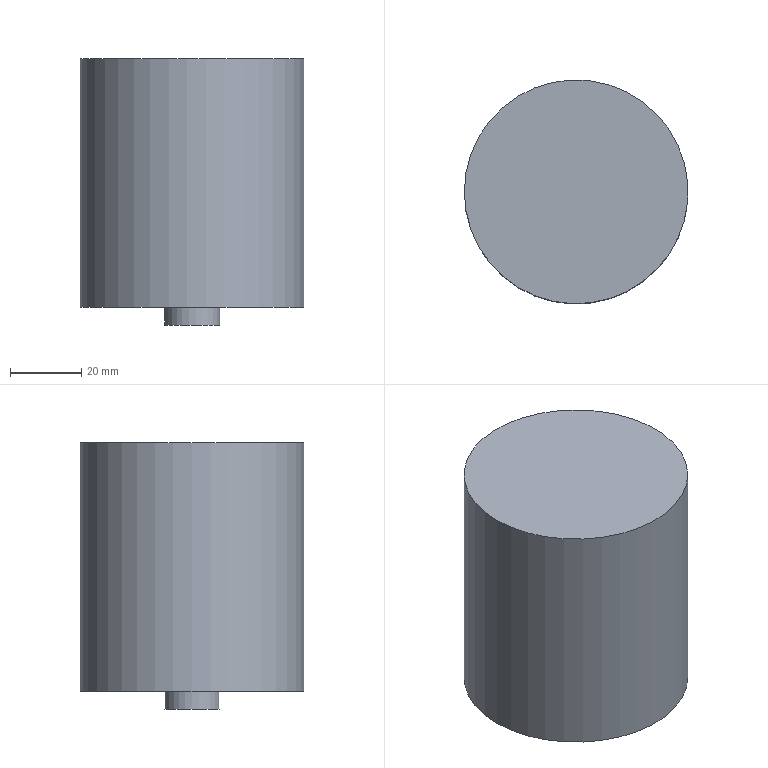Part | NX | features solid 2 | 1 solid | 5 faces | box 63 x 63 x 75 mm | volume 219151 mm3 | plane 3 | cylinder 2 | commonest cylinder face diameters 15.5 x1 63 x1
STEP:
#1=CARTESIAN_POINT('',(1202.,-543.5,-180.));
#2=VERTEX_POINT('',#1);
#3=CARTESIAN_POINT('',(1233.5,-543.5,-180.));
#4=DIRECTION('',(0.,0.,1.));
#5=DIRECTION('',(-1.,0.,0.));
#6=AXIS2_PLACEMENT_3D('',#3,#4,#5);
#7=CIRCLE('',#6,31.5);
#8=EDGE_CURVE('',#2,#2,#7,.T.);
#9=ORIENTED_EDGE('',*,*,#8,.F.);
#10=EDGE_LOOP('',(#9));
#11=FACE_BOUND('',#10,.T.);
#12=CARTESIAN_POINT('',(1225.75,-543.5,-180.));
#13=VERTEX_POINT('',#12);
#14=CARTESIAN_POINT('',(1233.5,-543.5,-180.));
#15=DIRECTION('',(0.,0.,1.));
#16=DIRECTION('',(-1.,0.,0.));
#17=AXIS2_PLACEMENT_3D('',#14,#15,#16);
#18=CIRCLE('',#17,7.75);
#19=EDGE_CURVE('',#13,#13,#18,.F.);
#20=ORIENTED_EDGE('',*,*,#19,.F.);
#21=EDGE_LOOP('',(#20));
#22=FACE_BOUND('',#21,.T.);
#23=CARTESIAN_POINT('',(1233.5,-543.5,-180.));
#24=DIRECTION('',(0.,0.,1.));
#25=DIRECTION('',(-1.,0.,0.));
#26=AXIS2_PLACEMENT_3D('',#23,#24,#25);
#27=PLANE('',#26);
#28=ADVANCED_FACE('',(#11,#22),#27,.F.);
#29=ORIENTED_EDGE('',*,*,#8,.T.);
#30=EDGE_LOOP('',(#29));
#31=FACE_BOUND('',#30,.T.);
#32=CARTESIAN_POINT('',(1202.,-543.5,-110.));
#33=VERTEX_POINT('',#32);
#34=CARTESIAN_POINT('',(1233.5,-543.5,-110.));
#35=DIRECTION('',(0.,0.,-1.));
#36=DIRECTION('',(-1.,0.,0.));
#37=AXIS2_PLACEMENT_3D('',#34,#35,#36);
#38=CIRCLE('',#37,31.5);
#39=EDGE_CURVE('',#33,#33,#38,.F.);
#40=ORIENTED_EDGE('',*,*,#39,.F.);
#41=EDGE_LOOP('',(#40));
#42=FACE_BOUND('',#41,.T.);
#43=CARTESIAN_POINT('',(1233.5,-543.5,-180.));
#44=DIRECTION('',(0.,0.,1.));
#45=DIRECTION('',(-1.,0.,0.));
#46=AXIS2_PLACEMENT_3D('',#43,#44,#45);
#47=CYLINDRICAL_SURFACE('',#46,31.5);
#48=ADVANCED_FACE('',(#31,#42),#47,.T.);
#49=ORIENTED_EDGE('',*,*,#39,.T.);
#50=EDGE_LOOP('',(#49));
#51=FACE_BOUND('',#50,.T.);
#52=CARTESIAN_POINT('',(1233.5,-543.5,-110.));
#53=DIRECTION('',(0.,0.,1.));
#54=DIRECTION('',(-1.,0.,0.));
#55=AXIS2_PLACEMENT_3D('',#52,#53,#54);
#56=PLANE('',#55);
#57=ADVANCED_FACE('',(#51),#56,.T.);
#58=ORIENTED_EDGE('',*,*,#19,.T.);
#59=EDGE_LOOP('',(#58));
#60=FACE_BOUND('',#59,.T.);
#61=CARTESIAN_POINT('',(1225.75,-543.5,-185.));
#62=VERTEX_POINT('',#61);
#63=CARTESIAN_POINT('',(1233.5,-543.5,-185.));
#64=DIRECTION('',(0.,0.,1.));
#65=DIRECTION('',(-1.,0.,0.));
#66=AXIS2_PLACEMENT_3D('',#63,#64,#65);
#67=CIRCLE('',#66,7.75);
#68=EDGE_CURVE('',#62,#62,#67,.T.);
#69=ORIENTED_EDGE('',*,*,#68,.T.);
#70=EDGE_LOOP('',(#69));
#71=FACE_BOUND('',#70,.T.);
#72=CARTESIAN_POINT('',(1233.5,-543.5,-180.));
#73=DIRECTION('',(0.,0.,-1.));
#74=DIRECTION('',(1.,0.,0.));
#75=AXIS2_PLACEMENT_3D('',#72,#73,#74);
#76=CYLINDRICAL_SURFACE('',#75,7.75);
#77=ADVANCED_FACE('',(#60,#71),#76,.T.);
#78=ORIENTED_EDGE('',*,*,#68,.F.);
#79=EDGE_LOOP('',(#78));
#80=FACE_BOUND('',#79,.T.);
#81=CARTESIAN_POINT('',(1233.5,-543.5,-185.));
#82=DIRECTION('',(0.,0.,1.));
#83=DIRECTION('',(-1.,0.,0.));
#84=AXIS2_PLACEMENT_3D('',#81,#82,#83);
#85=PLANE('',#84);
#86=ADVANCED_FACE('',(#80),#85,.F.);
#87=CLOSED_SHELL('',(#28,#48,#57,#77,#86));
#88=MANIFOLD_SOLID_BREP('',#87);
#89=(LENGTH_UNIT()NAMED_UNIT(*)SI_UNIT(.MILLI.,.METRE.));
#90=UNCERTAINTY_MEASURE_WITH_UNIT(LENGTH_MEASURE(0.00001),#89,'','');
#91=(NAMED_UNIT(*)PLANE_ANGLE_UNIT()SI_UNIT($,.RADIAN.));
#92=(NAMED_UNIT(*)SI_UNIT($,.STERADIAN.)SOLID_ANGLE_UNIT());
#93=(GEOMETRIC_REPRESENTATION_CONTEXT(3)GLOBAL_UNCERTAINTY_ASSIGNED_CONTEXT((#90))GLOBAL_UNIT_ASSIGNED_CONTEXT((#89,#91,#92))REPRESENTATION_CONTEXT('',''));
#94=ADVANCED_BREP_SHAPE_REPRESENTATION('',(#88),#93);